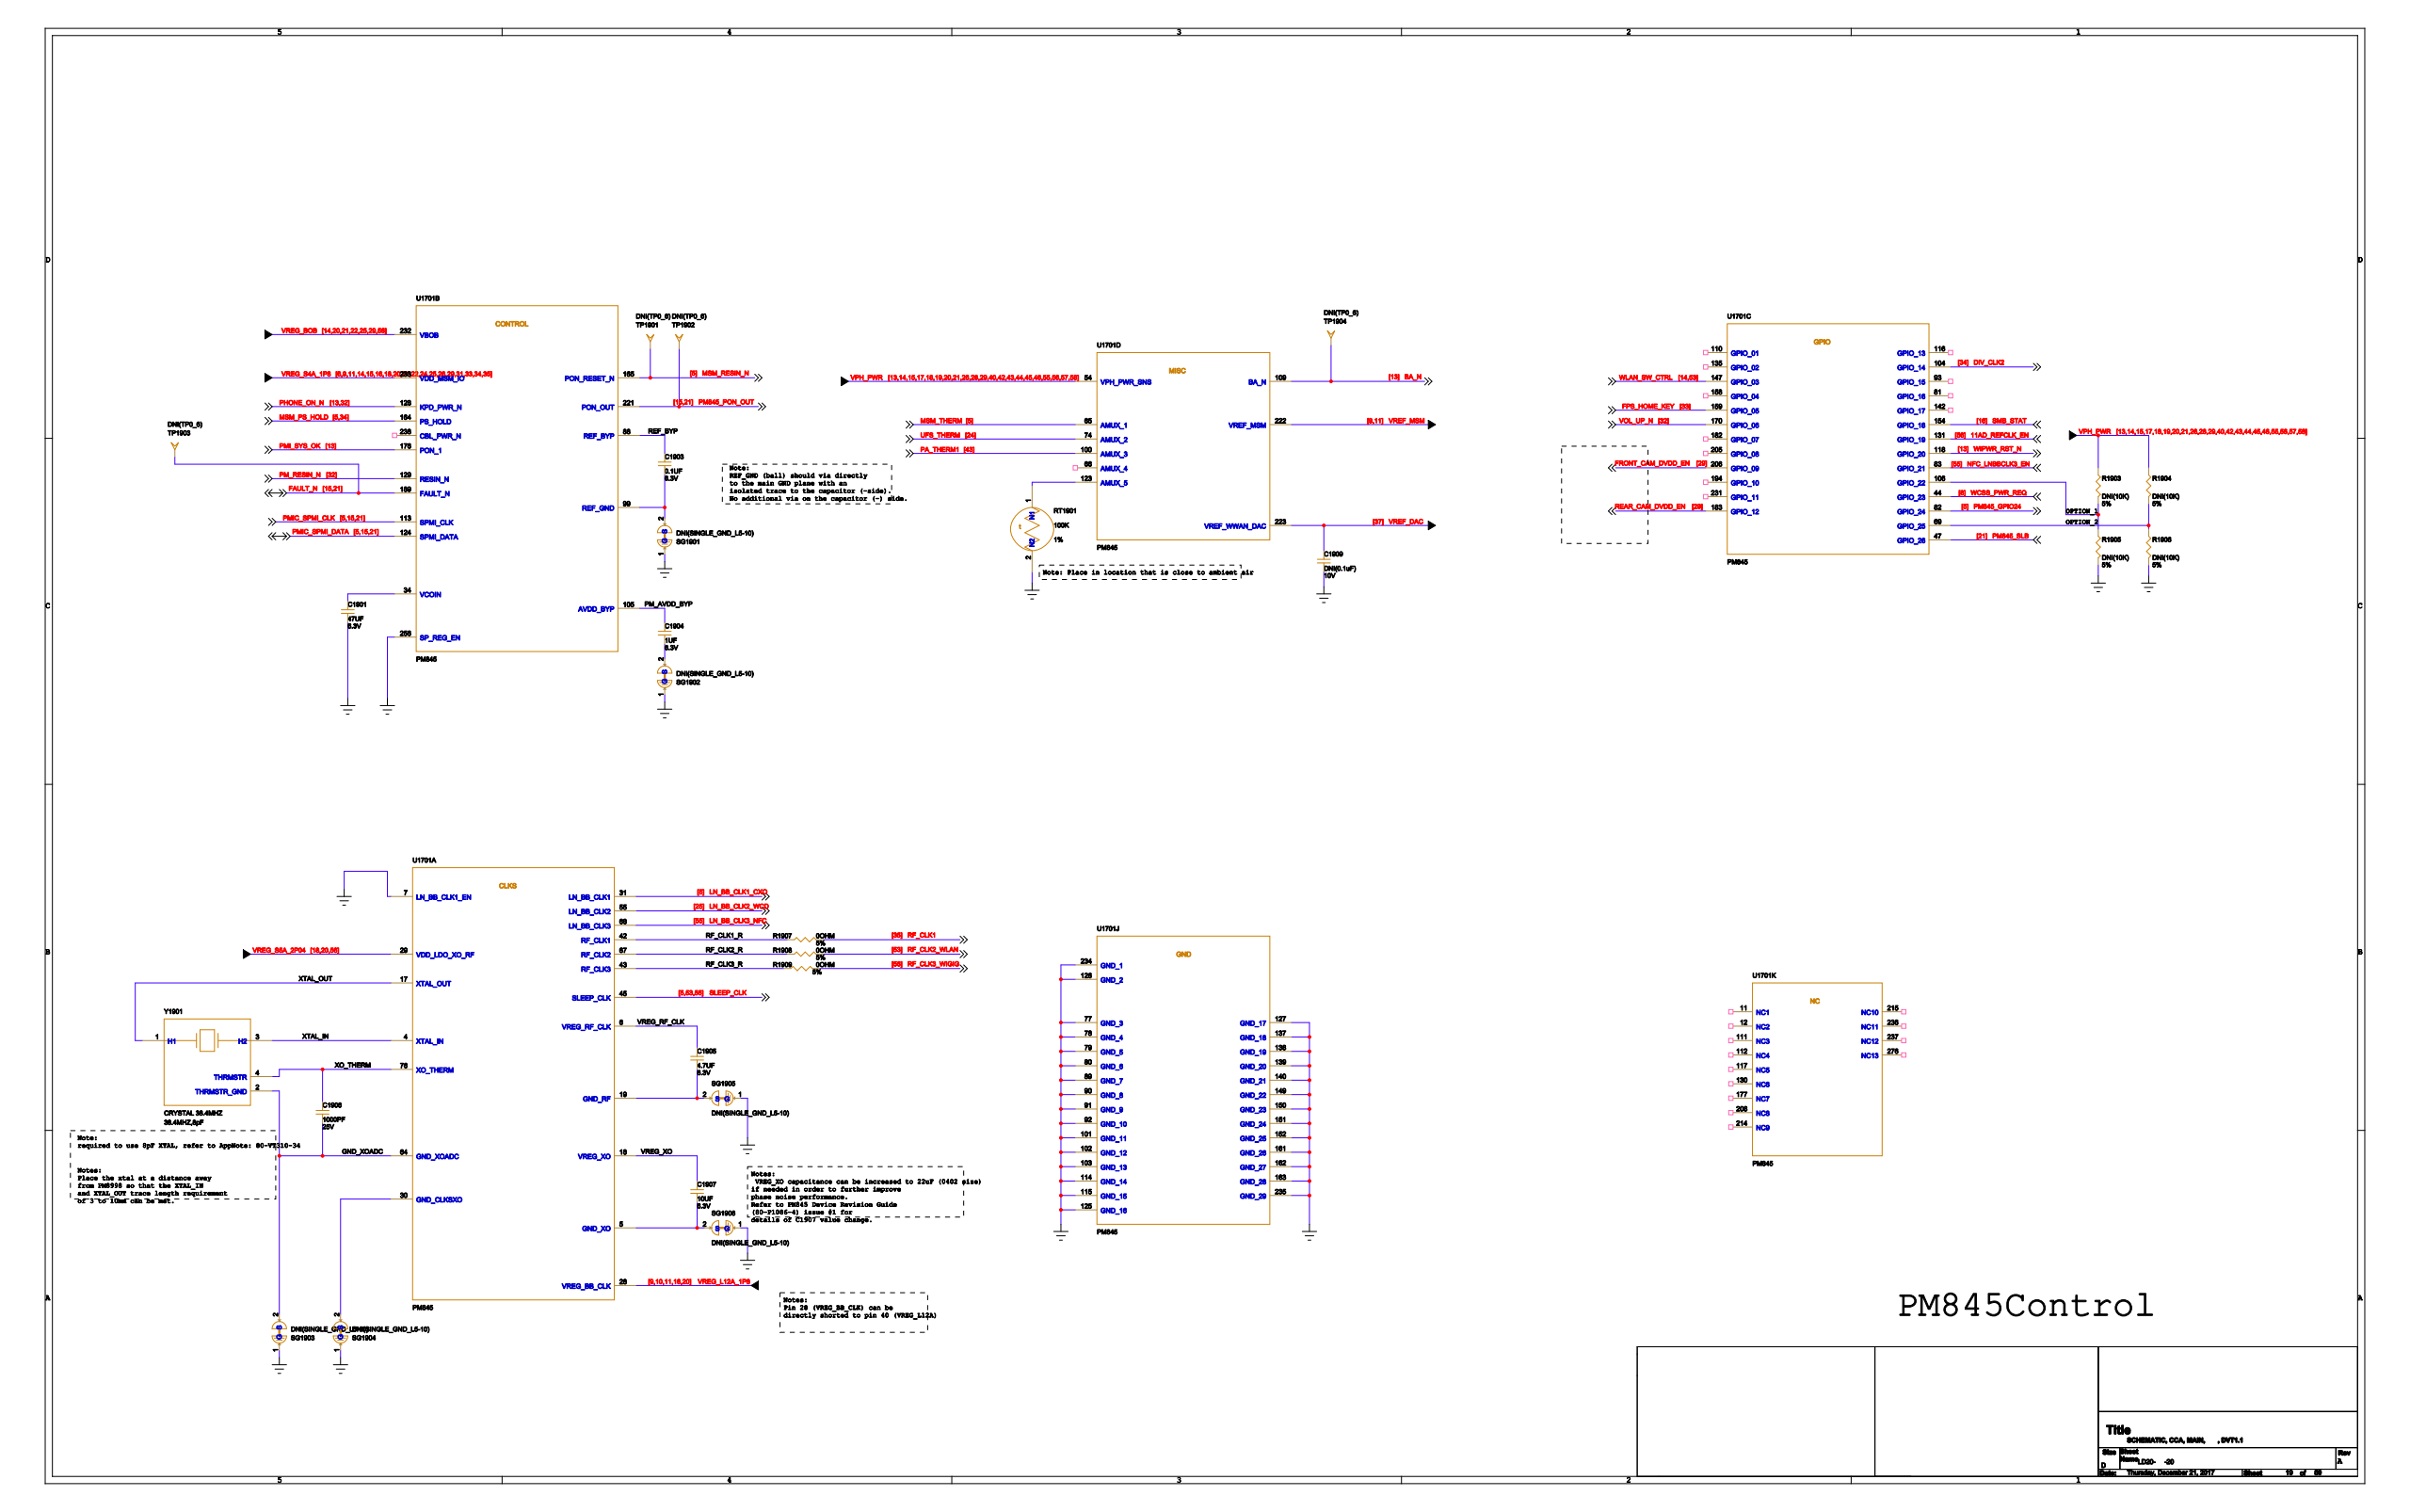Circuit board | Cadence Allegro | 1520 parts | 1149 nets | one sheet of the schematic
Parts on this sheet (reference | value | footprint):
C1901 | 47UF | 2P0603R
C1903 | 0.1UF | 2P0201R
C1904 | 1UF | 2P0201R
C1905 | 4.7UF | 2P0402R
C1906 | 1000PF | 2P0201R
C1907 | 10UF | 2P0402RV1
C1909 | DNI(0.1uF) | 2P0201R_DNI
R1903 | DNI(10K) | 2P0201R_DNI
R1904 | DNI(10K) | 2P0201R_DNI
R1905 | DNI(10K) | 2P0201R_DNI
R1906 | DNI(10K) | 2P0201R_DNI
R1907 | 0OHM | 2P0201R
R1908 | 0OHM | 2P0201R
R1909 | 0OHM | 2P0201R
RT1901 | 100K | 2P0201R
SG1901 | DNI(SINGLE_GND_L5-10) | GND_L5-10
SG1902 | DNI(SINGLE_GND_L5-10) | GND_L5-10
SG1903 | DNI(SINGLE_GND_L5-10) | GND_L5-10
SG1904 | DNI(SINGLE_GND_L5-10) | GND_L5-10
SG1905 | DNI(SINGLE_GND_L5-10) | GND_L5-10
SG1906 | DNI(SINGLE_GND_L5-10) | GND_L5-10
TP1901 | DNI(TP0_6) | TP-0_6
TP1902 | DNI(TP0_6) | TP-0_6
TP1903 | DNI(TP0_6) | TP-0_6
TP1904 | DNI(TP0_6) | TP-0_6
U1701 | PM845 | 287PGA242X240B138D45
Y1901 | CRYSTAL 38.4MHZ | 4PSM67X51NV1
Nets of these parts (net: part-pin ...):
GND: C1901-2 C1909-2 R1905-1 R1906-1 RT1901-2 SG1901-1 SG1902-1 SG1903-1 SG1904-1 SG1905-1 SG1906-1 U1701-7 U1701-77 U1701-78 U1701-79 U1701-80 U1701-89 U1701-90 U1701-91 U1701-92 U1701-101 U1701-102 U1701-103 U1701-114 U1701-115 U1701-125 U1701-126 U1701-127 U1701-137 U1701-138 U1701-139 U1701-140 U1701-149 U1701-150 U1701-151 U1701-152 U1701-161 U1701-162 U1701-163 U1701-234 U1701-235 U1701-256
VREG_BOB: U1701-1 U1701-14 U1701-232
VREG_S4A_1P8: U1701-57 U1701-233
N34054928: C1903-2 SG1901-2 U1701-99
N34054956: C1904-2 SG1902-2
GND_XOADC: C1906-2 SG1903-2 Y1901-2 U1701-64
N34056315: SG1904-2 U1701-30
N34056642: C1905-2 SG1905-2 U1701-19
N34056734: C1907-2 SG1906-2 U1701-5
VREG_S5A_2P04: U1701-29
SLEEP_CLK: U1701-45
11AD_REFCLK_EN: U1701-131
RF_CLK3_WIGIG: R1909-1
VPH_PWR: R1903-2 R1904-2 U1701-54 U1701-56
MSM_RESIN_N: TP1901-1 U1701-165
NFC_LNBBCLK3_EN: U1701-83
LN_BB_CLK2_WCD: U1701-55
REAR_CAM_DVDD_EN: U1701-183
FRONT_CAM_DVDD_EN: U1701-206
XTAL_OUT: Y1901-1 U1701-17
XTAL_IN: Y1901-3 U1701-4
XO_THERM: C1906-1 Y1901-4 U1701-76
SMB_STAT: U1701-154
VREG_L12A_1P8: U1701-28 U1701-40
VREF_DAC: C1909-1 U1701-223
VREF_MSM: U1701-222
REF_BYP: C1903-1 U1701-88
PM_AVDD_BYP: C1904-1 U1701-105
VREG_RF_CLK: C1905-1 U1701-6
VREG_XO: C1907-1 U1701-18
N34054785: C1901-1 U1701-34
PA_THERM1: U1701-100
RF_CLK2_WLAN: R1908-1
LN_BB_CLK3_NFC: U1701-68
RF_CLK1: R1907-1
RF_CLK1_R: R1907-2 U1701-42
RF_CLK2_R: R1908-2 U1701-67
RF_CLK3_R: R1909-2 U1701-43
FPS_HOME_KEY: U1701-159
MSM_PS_HOLD: U1701-164
PM845_GPIO24: U1701-82
N34055728: R1903-1 R1905-2 U1701-106
N34055758: R1904-1 R1906-2 U1701-69
WIPWR_RST_N: U1701-118
VOL_UP_N: U1701-170
PM_RESIN_N: U1701-129
PHONE_ON_N: U1701-128
UFS_THERM: U1701-74
MSM_THERM: U1701-65
N34055117: RT1901-1 U1701-123
BA_N: TP1904-1 U1701-109
PMIC_SPMI_DATA: U1701-124
PMIC_SPMI_CLK: U1701-113
DIV_CLK2: U1701-104
FAULT_N: TP1903-1 U1701-189
LN_BB_CLK1_CXO: U1701-31
PM845_PON_OUT: TP1902-1 U1701-221
PM845_SLB: U1701-47
WCSS_PWR_REQ: U1701-44
PMI_SYS_OK: U1701-176
WLAN_SW_CTRL: U1701-147